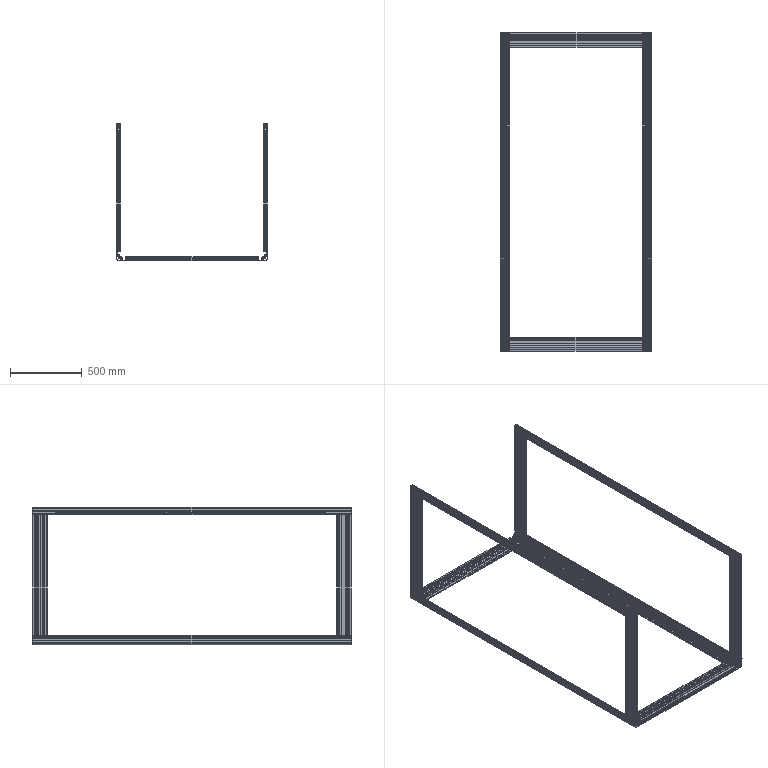Part | 13 solids | 1101 faces | box 1050 x 2216 x 955 mm | volume 10793369 mm3 | plane 770 | cylinder 331 | commonest cylinder face diameters 0.6 x80 0.4 x63 15 x48 2 x20 0.24 x18 9 x18